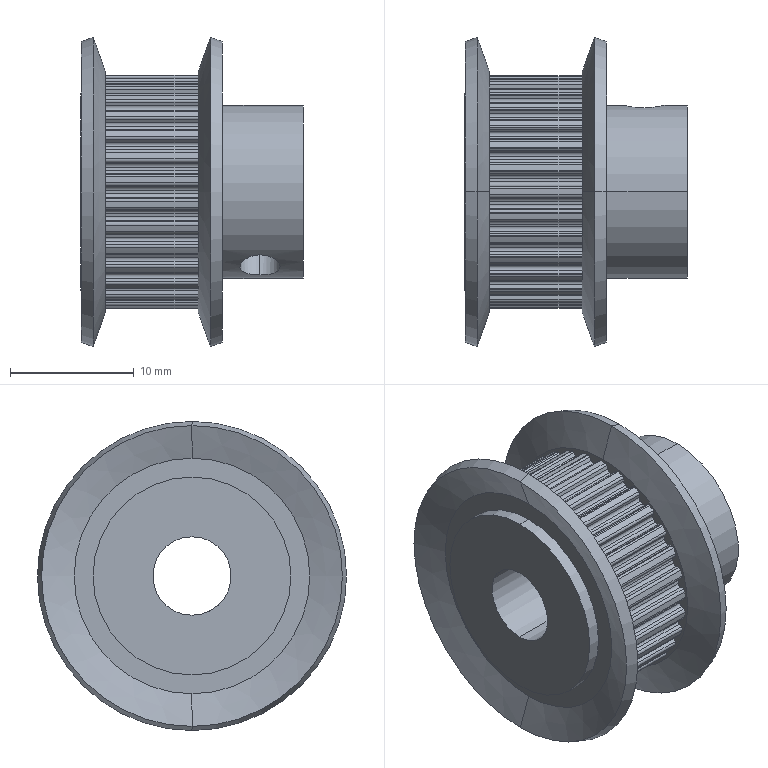Part | STEP file | ATP30MXL025-B-P6.35 | 1 solid | 296 faces | box 18 x 25 x 25 mm | volume 3723 mm3 | cylinder 217 | plane 67 | cone 12 | commonest cylinder face diameters 0.46 x72 0.6 x72 18.9 x31 17.62 x30 3.242 x4 16 x4